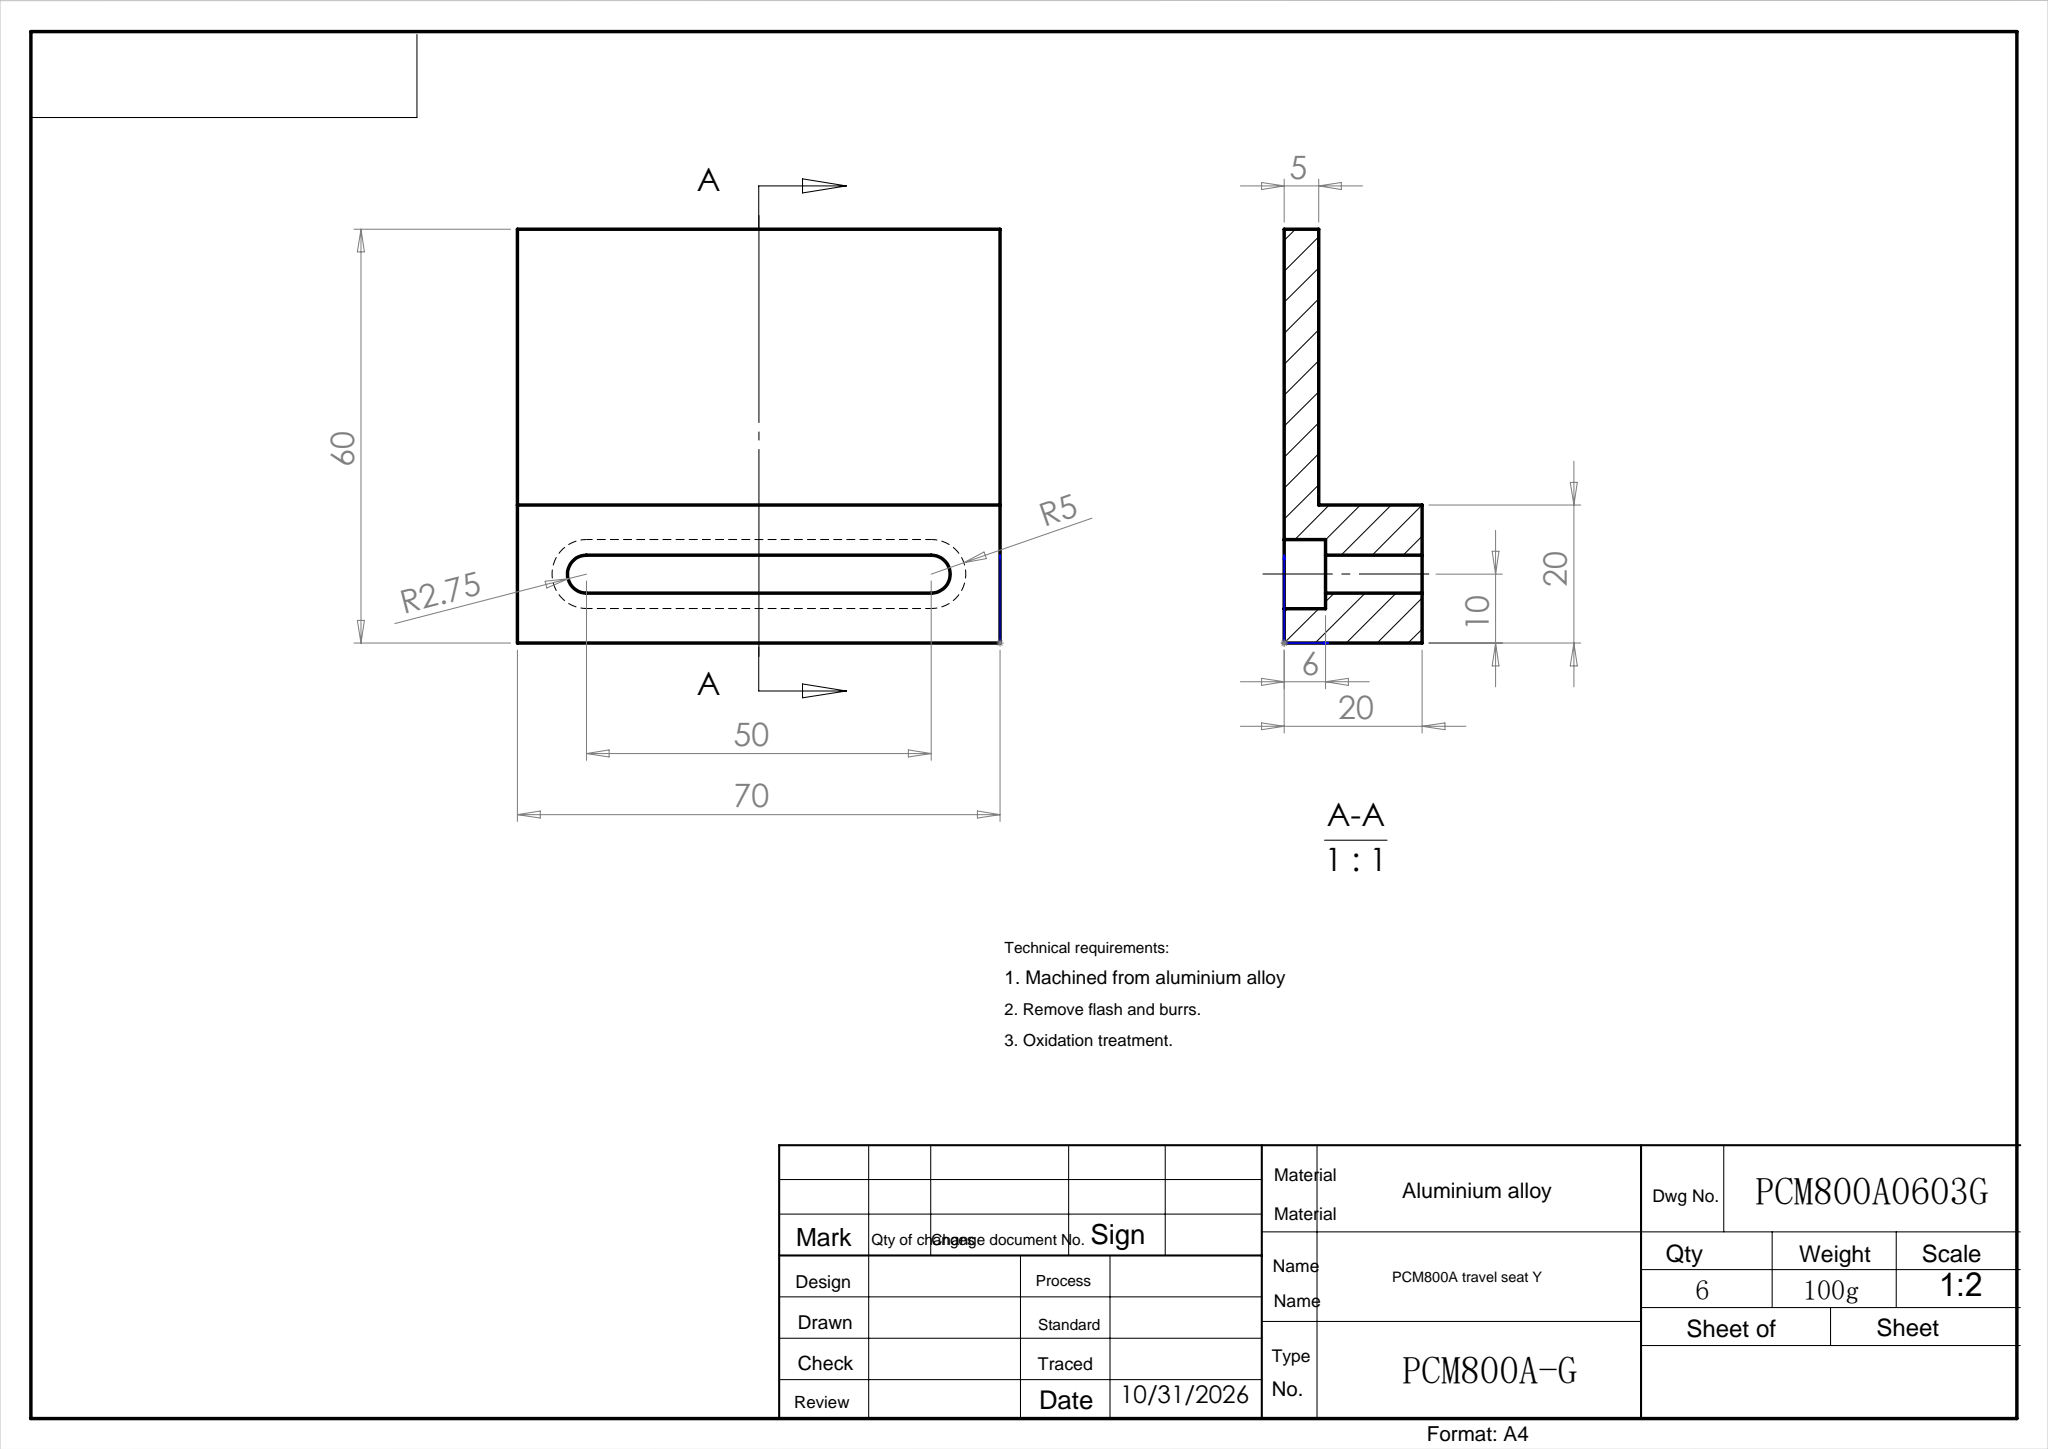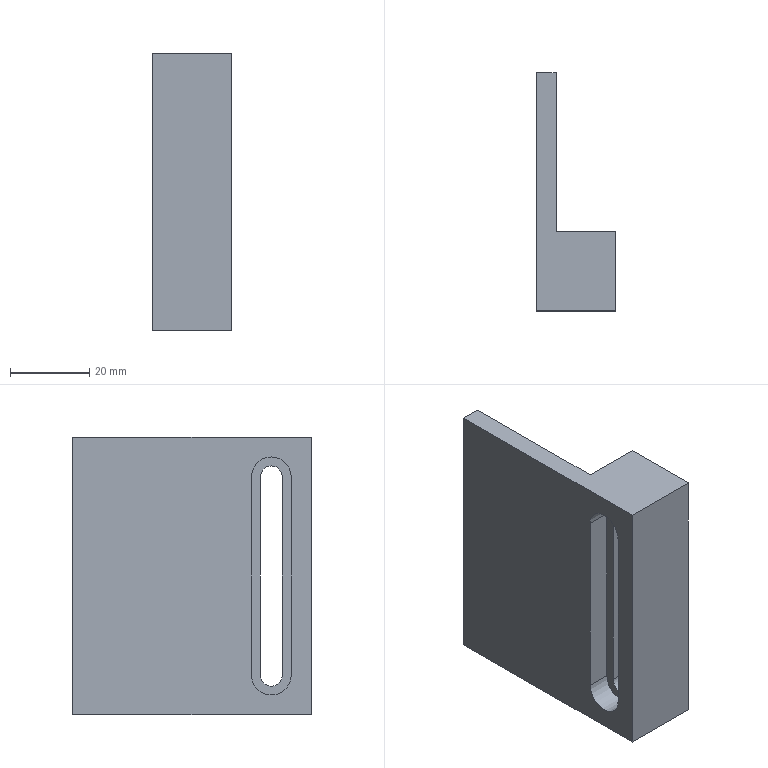Part | SolidWorks | features ICE 2, Extrusion 1 | 1 solid | 19 faces | box 20 x 60 x 70 mm | volume 34346 mm3 | plane 13 | cylinder 6 | commonest cylinder face diameters 5.5 x3 10 x3
STEP:
#1=CARTESIAN_POINT('',(6.,10.,65.));
#2=VERTEX_POINT('',#1);
#3=CARTESIAN_POINT('',(6.,15.,60.));
#4=VERTEX_POINT('',#3);
#5=CARTESIAN_POINT('',(6.,10.,60.));
#6=DIRECTION('',(-1.,0.,0.));
#7=DIRECTION('',(0.,0.,1.));
#8=AXIS2_PLACEMENT_3D('',#5,#6,#7);
#9=CIRCLE('',#8,5.);
#10=EDGE_CURVE('',#2,#4,#9,.T.);
#11=ORIENTED_EDGE('',*,*,#10,.F.);
#12=CARTESIAN_POINT('',(0.,10.,65.));
#13=VERTEX_POINT('',#12);
#14=CARTESIAN_POINT('',(6.,10.,65.));
#15=DIRECTION('',(-1.,0.,0.));
#16=VECTOR('',#15,1000.);
#17=LINE('',#14,#16);
#18=EDGE_CURVE('',#2,#13,#17,.T.);
#19=ORIENTED_EDGE('',*,*,#18,.T.);
#20=CARTESIAN_POINT('',(0.,15.,60.));
#21=VERTEX_POINT('',#20);
#22=CARTESIAN_POINT('',(0.,10.,60.));
#23=DIRECTION('',(-1.,0.,0.));
#24=DIRECTION('',(0.,0.,1.));
#25=AXIS2_PLACEMENT_3D('',#22,#23,#24);
#26=CIRCLE('',#25,5.);
#27=EDGE_CURVE('',#13,#21,#26,.T.);
#28=ORIENTED_EDGE('',*,*,#27,.T.);
#29=CARTESIAN_POINT('',(6.,15.,60.));
#30=DIRECTION('',(-1.,0.,0.));
#31=VECTOR('',#30,1000.);
#32=LINE('',#29,#31);
#33=EDGE_CURVE('',#4,#21,#32,.T.);
#34=ORIENTED_EDGE('',*,*,#33,.F.);
#35=EDGE_LOOP('',(#11,#19,#28,#34));
#36=FACE_OUTER_BOUND('',#35,.T.);
#37=CARTESIAN_POINT('',(6.,10.,60.));
#38=DIRECTION('',(-1.,0.,0.));
#39=DIRECTION('',(0.,0.,1.));
#40=AXIS2_PLACEMENT_3D('',#37,#38,#39);
#41=CYLINDRICAL_SURFACE('',#40,5.);
#42=ADVANCED_FACE('',(#36),#41,.F.);
#43=CARTESIAN_POINT('',(20.,10.,62.75));
#44=VERTEX_POINT('',#43);
#45=CARTESIAN_POINT('',(20.,12.75,60.));
#46=VERTEX_POINT('',#45);
#47=CARTESIAN_POINT('',(20.,10.,60.));
#48=DIRECTION('',(-1.,0.,0.));
#49=DIRECTION('',(0.,-1.,0.));
#50=AXIS2_PLACEMENT_3D('',#47,#48,#49);
#51=CIRCLE('',#50,2.75);
#52=EDGE_CURVE('',#44,#46,#51,.T.);
#53=ORIENTED_EDGE('',*,*,#52,.F.);
#54=CARTESIAN_POINT('',(6.,10.,62.75));
#55=VERTEX_POINT('',#54);
#56=CARTESIAN_POINT('',(1200.,10.,62.75));
#57=DIRECTION('',(-1.,0.,0.));
#58=VECTOR('',#57,1000.);
#59=LINE('',#56,#58);
#60=EDGE_CURVE('',#44,#55,#59,.T.);
#61=ORIENTED_EDGE('',*,*,#60,.T.);
#62=CARTESIAN_POINT('',(6.,12.75,60.));
#63=VERTEX_POINT('',#62);
#64=CARTESIAN_POINT('',(6.,10.,60.));
#65=DIRECTION('',(1.,0.,0.));
#66=DIRECTION('',(0.,0.,1.));
#67=AXIS2_PLACEMENT_3D('',#64,#65,#66);
#68=CIRCLE('',#67,2.75);
#69=EDGE_CURVE('',#63,#55,#68,.T.);
#70=ORIENTED_EDGE('',*,*,#69,.F.);
#71=CARTESIAN_POINT('',(1200.,12.75,60.));
#72=DIRECTION('',(-1.,0.,0.));
#73=VECTOR('',#72,1000.);
#74=LINE('',#71,#73);
#75=EDGE_CURVE('',#46,#63,#74,.T.);
#76=ORIENTED_EDGE('',*,*,#75,.F.);
#77=EDGE_LOOP('',(#53,#61,#70,#76));
#78=FACE_OUTER_BOUND('',#77,.T.);
#79=CARTESIAN_POINT('',(1200.,10.,60.));
#80=DIRECTION('',(-1.,0.,0.));
#81=DIRECTION('',(0.,0.,1.));
#82=AXIS2_PLACEMENT_3D('',#79,#80,#81);
#83=CYLINDRICAL_SURFACE('',#82,2.75);
#84=ADVANCED_FACE('',(#78),#83,.F.);
#85=CARTESIAN_POINT('',(6.,7.25,10.));
#86=VERTEX_POINT('',#85);
#87=CARTESIAN_POINT('',(6.,12.75,10.));
#88=VERTEX_POINT('',#87);
#89=CARTESIAN_POINT('',(6.,10.,10.));
#90=DIRECTION('',(1.,0.,0.));
#91=DIRECTION('',(0.,0.,1.));
#92=AXIS2_PLACEMENT_3D('',#89,#90,#91);
#93=CIRCLE('',#92,2.75);
#94=EDGE_CURVE('',#86,#88,#93,.T.);
#95=ORIENTED_EDGE('',*,*,#94,.F.);
#96=CARTESIAN_POINT('',(20.,7.25,10.));
#97=VERTEX_POINT('',#96);
#98=CARTESIAN_POINT('',(1200.,7.25,10.));
#99=DIRECTION('',(-1.,0.,0.));
#100=VECTOR('',#99,1000.);
#101=LINE('',#98,#100);
#102=EDGE_CURVE('',#97,#86,#101,.T.);
#103=ORIENTED_EDGE('',*,*,#102,.F.);
#104=CARTESIAN_POINT('',(20.,12.75,10.));
#105=VERTEX_POINT('',#104);
#106=CARTESIAN_POINT('',(20.,10.,10.));
#107=DIRECTION('',(-1.,0.,0.));
#108=DIRECTION('',(0.,-1.,0.));
#109=AXIS2_PLACEMENT_3D('',#106,#107,#108);
#110=CIRCLE('',#109,2.75);
#111=EDGE_CURVE('',#105,#97,#110,.T.);
#112=ORIENTED_EDGE('',*,*,#111,.F.);
#113=CARTESIAN_POINT('',(1200.,12.75,10.));
#114=DIRECTION('',(-1.,0.,0.));
#115=VECTOR('',#114,1000.);
#116=LINE('',#113,#115);
#117=EDGE_CURVE('',#105,#88,#116,.T.);
#118=ORIENTED_EDGE('',*,*,#117,.T.);
#119=EDGE_LOOP('',(#95,#103,#112,#118));
#120=FACE_OUTER_BOUND('',#119,.T.);
#121=CARTESIAN_POINT('',(1200.,10.,10.));
#122=DIRECTION('',(-1.,0.,0.));
#123=DIRECTION('',(0.,0.,1.));
#124=AXIS2_PLACEMENT_3D('',#121,#122,#123);
#125=CYLINDRICAL_SURFACE('',#124,2.75);
#126=ADVANCED_FACE('',(#120),#125,.F.);
#127=CARTESIAN_POINT('',(6.,12.75,10.));
#128=DIRECTION('',(0.,0.,1.));
#129=VECTOR('',#128,1000.);
#130=LINE('',#127,#129);
#131=EDGE_CURVE('',#88,#63,#130,.T.);
#132=ORIENTED_EDGE('',*,*,#131,.F.);
#133=ORIENTED_EDGE('',*,*,#117,.F.);
#134=CARTESIAN_POINT('',(20.,12.75,70.));
#135=DIRECTION('',(0.,0.,-1.));
#136=VECTOR('',#135,1000.);
#137=LINE('',#134,#136);
#138=EDGE_CURVE('',#46,#105,#137,.T.);
#139=ORIENTED_EDGE('',*,*,#138,.F.);
#140=ORIENTED_EDGE('',*,*,#75,.T.);
#141=EDGE_LOOP('',(#132,#133,#139,#140));
#142=FACE_OUTER_BOUND('',#141,.T.);
#143=CARTESIAN_POINT('',(1200.,12.75,10.));
#144=DIRECTION('',(0.,1.,0.));
#145=DIRECTION('',(0.,0.,1.));
#146=AXIS2_PLACEMENT_3D('',#143,#144,#145);
#147=PLANE('',#146);
#148=ADVANCED_FACE('',(#142),#147,.F.);
#149=ORIENTED_EDGE('',*,*,#60,.F.);
#150=CARTESIAN_POINT('',(20.,7.25,60.));
#151=VERTEX_POINT('',#150);
#152=CARTESIAN_POINT('',(20.,10.,60.));
#153=DIRECTION('',(-1.,0.,0.));
#154=DIRECTION('',(0.,-1.,0.));
#155=AXIS2_PLACEMENT_3D('',#152,#153,#154);
#156=CIRCLE('',#155,2.75);
#157=EDGE_CURVE('',#151,#44,#156,.T.);
#158=ORIENTED_EDGE('',*,*,#157,.F.);
#159=CARTESIAN_POINT('',(6.,7.25,60.));
#160=VERTEX_POINT('',#159);
#161=CARTESIAN_POINT('',(1200.,7.25,60.));
#162=DIRECTION('',(-1.,0.,0.));
#163=VECTOR('',#162,1000.);
#164=LINE('',#161,#163);
#165=EDGE_CURVE('',#151,#160,#164,.T.);
#166=ORIENTED_EDGE('',*,*,#165,.T.);
#167=CARTESIAN_POINT('',(6.,10.,60.));
#168=DIRECTION('',(1.,0.,0.));
#169=DIRECTION('',(0.,0.,1.));
#170=AXIS2_PLACEMENT_3D('',#167,#168,#169);
#171=CIRCLE('',#170,2.75);
#172=EDGE_CURVE('',#55,#160,#171,.T.);
#173=ORIENTED_EDGE('',*,*,#172,.F.);
#174=EDGE_LOOP('',(#149,#158,#166,#173));
#175=FACE_OUTER_BOUND('',#174,.T.);
#176=CARTESIAN_POINT('',(1200.,10.,60.));
#177=DIRECTION('',(-1.,0.,0.));
#178=DIRECTION('',(0.,0.,1.));
#179=AXIS2_PLACEMENT_3D('',#176,#177,#178);
#180=CYLINDRICAL_SURFACE('',#179,2.75);
#181=ADVANCED_FACE('',(#175),#180,.F.);
#182=CARTESIAN_POINT('',(6.,7.25,10.));
#183=DIRECTION('',(0.,0.,-1.));
#184=VECTOR('',#183,1000.);
#185=LINE('',#182,#184);
#186=EDGE_CURVE('',#160,#86,#185,.T.);
#187=ORIENTED_EDGE('',*,*,#186,.F.);
#188=ORIENTED_EDGE('',*,*,#165,.F.);
#189=CARTESIAN_POINT('',(20.,7.25,70.));
#190=DIRECTION('',(0.,0.,1.));
#191=VECTOR('',#190,1000.);
#192=LINE('',#189,#191);
#193=EDGE_CURVE('',#97,#151,#192,.T.);
#194=ORIENTED_EDGE('',*,*,#193,.F.);
#195=ORIENTED_EDGE('',*,*,#102,.T.);
#196=EDGE_LOOP('',(#187,#188,#194,#195));
#197=FACE_OUTER_BOUND('',#196,.T.);
#198=CARTESIAN_POINT('',(1200.,7.25,10.));
#199=DIRECTION('',(0.,-1.,0.));
#200=DIRECTION('',(0.,0.,-1.));
#201=AXIS2_PLACEMENT_3D('',#198,#199,#200);
#202=PLANE('',#201);
#203=ADVANCED_FACE('',(#197),#202,.F.);
#204=CARTESIAN_POINT('',(0.,0.,0.));
#205=VERTEX_POINT('',#204);
#206=CARTESIAN_POINT('',(20.,0.,0.));
#207=VERTEX_POINT('',#206);
#208=CARTESIAN_POINT('',(20.,0.,0.));
#209=DIRECTION('',(1.,0.,0.));
#210=VECTOR('',#209,1000.);
#211=LINE('',#208,#210);
#212=EDGE_CURVE('',#205,#207,#211,.T.);
#213=ORIENTED_EDGE('',*,*,#212,.T.);
#214=CARTESIAN_POINT('',(20.,0.,70.));
#215=VERTEX_POINT('',#214);
#216=CARTESIAN_POINT('',(20.,0.,70.));
#217=DIRECTION('',(0.,0.,-1.));
#218=VECTOR('',#217,1000.);
#219=LINE('',#216,#218);
#220=EDGE_CURVE('',#215,#207,#219,.T.);
#221=ORIENTED_EDGE('',*,*,#220,.F.);
#222=CARTESIAN_POINT('',(0.,0.,70.));
#223=VERTEX_POINT('',#222);
#224=CARTESIAN_POINT('',(20.,0.,70.));
#225=DIRECTION('',(1.,0.,0.));
#226=VECTOR('',#225,1000.);
#227=LINE('',#224,#226);
#228=EDGE_CURVE('',#223,#215,#227,.T.);
#229=ORIENTED_EDGE('',*,*,#228,.F.);
#230=CARTESIAN_POINT('',(0.,0.,70.));
#231=DIRECTION('',(0.,0.,-1.));
#232=VECTOR('',#231,1000.);
#233=LINE('',#230,#232);
#234=EDGE_CURVE('',#223,#205,#233,.T.);
#235=ORIENTED_EDGE('',*,*,#234,.T.);
#236=EDGE_LOOP('',(#213,#221,#229,#235));
#237=FACE_OUTER_BOUND('',#236,.T.);
#238=CARTESIAN_POINT('',(20.,0.,70.));
#239=DIRECTION('',(0.,1.,0.));
#240=DIRECTION('',(0.,0.,1.));
#241=AXIS2_PLACEMENT_3D('',#238,#239,#240);
#242=PLANE('',#241);
#243=ADVANCED_FACE('',(#237),#242,.F.);
#244=ORIENTED_EDGE('',*,*,#138,.T.);
#245=ORIENTED_EDGE('',*,*,#111,.T.);
#246=ORIENTED_EDGE('',*,*,#193,.T.);
#247=ORIENTED_EDGE('',*,*,#157,.T.);
#248=ORIENTED_EDGE('',*,*,#52,.T.);
#249=EDGE_LOOP('',(#244,#245,#246,#247,#248));
#250=FACE_BOUND('',#249,.T.);
#251=CARTESIAN_POINT('',(20.,20.,0.));
#252=VERTEX_POINT('',#251);
#253=CARTESIAN_POINT('',(20.,20.,0.));
#254=DIRECTION('',(0.,1.,0.));
#255=VECTOR('',#254,1000.);
#256=LINE('',#253,#255);
#257=EDGE_CURVE('',#207,#252,#256,.T.);
#258=ORIENTED_EDGE('',*,*,#257,.T.);
#259=CARTESIAN_POINT('',(20.,20.,70.));
#260=VERTEX_POINT('',#259);
#261=CARTESIAN_POINT('',(20.,20.,70.));
#262=DIRECTION('',(0.,0.,-1.));
#263=VECTOR('',#262,1000.);
#264=LINE('',#261,#263);
#265=EDGE_CURVE('',#260,#252,#264,.T.);
#266=ORIENTED_EDGE('',*,*,#265,.F.);
#267=CARTESIAN_POINT('',(20.,20.,70.));
#268=DIRECTION('',(0.,1.,0.));
#269=VECTOR('',#268,1000.);
#270=LINE('',#267,#269);
#271=EDGE_CURVE('',#215,#260,#270,.T.);
#272=ORIENTED_EDGE('',*,*,#271,.F.);
#273=ORIENTED_EDGE('',*,*,#220,.T.);
#274=EDGE_LOOP('',(#258,#266,#272,#273));
#275=FACE_OUTER_BOUND('',#274,.T.);
#276=CARTESIAN_POINT('',(20.,20.,70.));
#277=DIRECTION('',(-1.,0.,0.));
#278=DIRECTION('',(0.,-1.,0.));
#279=AXIS2_PLACEMENT_3D('',#276,#277,#278);
#280=PLANE('',#279);
#281=ADVANCED_FACE('',(#250,#275),#280,.F.);
#282=CARTESIAN_POINT('',(5.,20.,0.));
#283=VERTEX_POINT('',#282);
#284=CARTESIAN_POINT('',(5.,20.,0.));
#285=DIRECTION('',(-1.,0.,0.));
#286=VECTOR('',#285,1000.);
#287=LINE('',#284,#286);
#288=EDGE_CURVE('',#252,#283,#287,.T.);
#289=ORIENTED_EDGE('',*,*,#288,.T.);
#290=CARTESIAN_POINT('',(5.,20.,70.));
#291=VERTEX_POINT('',#290);
#292=CARTESIAN_POINT('',(5.,20.,70.));
#293=DIRECTION('',(0.,0.,-1.));
#294=VECTOR('',#293,1000.);
#295=LINE('',#292,#294);
#296=EDGE_CURVE('',#291,#283,#295,.T.);
#297=ORIENTED_EDGE('',*,*,#296,.F.);
#298=CARTESIAN_POINT('',(5.,20.,70.));
#299=DIRECTION('',(-1.,0.,0.));
#300=VECTOR('',#299,1000.);
#301=LINE('',#298,#300);
#302=EDGE_CURVE('',#260,#291,#301,.T.);
#303=ORIENTED_EDGE('',*,*,#302,.F.);
#304=ORIENTED_EDGE('',*,*,#265,.T.);
#305=EDGE_LOOP('',(#289,#297,#303,#304));
#306=FACE_OUTER_BOUND('',#305,.T.);
#307=CARTESIAN_POINT('',(5.,20.,70.));
#308=DIRECTION('',(0.,-1.,0.));
#309=DIRECTION('',(0.,0.,-1.));
#310=AXIS2_PLACEMENT_3D('',#307,#308,#309);
#311=PLANE('',#310);
#312=ADVANCED_FACE('',(#306),#311,.F.);
#313=CARTESIAN_POINT('',(5.,60.,0.));
#314=VERTEX_POINT('',#313);
#315=CARTESIAN_POINT('',(5.,60.,0.));
#316=DIRECTION('',(0.,1.,0.));
#317=VECTOR('',#316,1000.);
#318=LINE('',#315,#317);
#319=EDGE_CURVE('',#283,#314,#318,.T.);
#320=ORIENTED_EDGE('',*,*,#319,.T.);
#321=CARTESIAN_POINT('',(5.,60.,70.));
#322=VERTEX_POINT('',#321);
#323=CARTESIAN_POINT('',(5.,60.,70.));
#324=DIRECTION('',(0.,0.,-1.));
#325=VECTOR('',#324,1000.);
#326=LINE('',#323,#325);
#327=EDGE_CURVE('',#322,#314,#326,.T.);
#328=ORIENTED_EDGE('',*,*,#327,.F.);
#329=CARTESIAN_POINT('',(5.,60.,70.));
#330=DIRECTION('',(0.,1.,0.));
#331=VECTOR('',#330,1000.);
#332=LINE('',#329,#331);
#333=EDGE_CURVE('',#291,#322,#332,.T.);
#334=ORIENTED_EDGE('',*,*,#333,.F.);
#335=ORIENTED_EDGE('',*,*,#296,.T.);
#336=EDGE_LOOP('',(#320,#328,#334,#335));
#337=FACE_OUTER_BOUND('',#336,.T.);
#338=CARTESIAN_POINT('',(5.,60.,70.));
#339=DIRECTION('',(-1.,0.,0.));
#340=DIRECTION('',(0.,-1.,0.));
#341=AXIS2_PLACEMENT_3D('',#338,#339,#340);
#342=PLANE('',#341);
#343=ADVANCED_FACE('',(#337),#342,.F.);
#344=CARTESIAN_POINT('',(0.,60.,0.));
#345=VERTEX_POINT('',#344);
#346=CARTESIAN_POINT('',(0.,60.,0.));
#347=DIRECTION('',(-1.,0.,0.));
#348=VECTOR('',#347,1000.);
#349=LINE('',#346,#348);
#350=EDGE_CURVE('',#314,#345,#349,.T.);
#351=ORIENTED_EDGE('',*,*,#350,.T.);
#352=CARTESIAN_POINT('',(0.,60.,70.));
#353=VERTEX_POINT('',#352);
#354=CARTESIAN_POINT('',(0.,60.,70.));
#355=DIRECTION('',(0.,0.,-1.));
#356=VECTOR('',#355,1000.);
#357=LINE('',#354,#356);
#358=EDGE_CURVE('',#353,#345,#357,.T.);
#359=ORIENTED_EDGE('',*,*,#358,.F.);
#360=CARTESIAN_POINT('',(0.,60.,70.));
#361=DIRECTION('',(-1.,0.,0.));
#362=VECTOR('',#361,1000.);
#363=LINE('',#360,#362);
#364=EDGE_CURVE('',#322,#353,#363,.T.);
#365=ORIENTED_EDGE('',*,*,#364,.F.);
#366=ORIENTED_EDGE('',*,*,#327,.T.);
#367=EDGE_LOOP('',(#351,#359,#365,#366));
#368=FACE_OUTER_BOUND('',#367,.T.);
#369=CARTESIAN_POINT('',(0.,60.,70.));
#370=DIRECTION('',(0.,-1.,0.));
#371=DIRECTION('',(0.,0.,-1.));
#372=AXIS2_PLACEMENT_3D('',#369,#370,#371);
#373=PLANE('',#372);
#374=ADVANCED_FACE('',(#368),#373,.F.);
#375=CARTESIAN_POINT('',(0.,5.,10.));
#376=VERTEX_POINT('',#375);
#377=CARTESIAN_POINT('',(0.,5.,60.));
#378=VERTEX_POINT('',#377);
#379=CARTESIAN_POINT('',(0.,5.,10.));
#380=DIRECTION('',(0.,0.,1.));
#381=VECTOR('',#380,1000.);
#382=LINE('',#379,#381);
#383=EDGE_CURVE('',#376,#378,#382,.T.);
#384=ORIENTED_EDGE('',*,*,#383,.F.);
#385=CARTESIAN_POINT('',(0.,15.,10.));
#386=VERTEX_POINT('',#385);
#387=CARTESIAN_POINT('',(0.,10.,10.));
#388=DIRECTION('',(-1.,0.,0.));
#389=DIRECTION('',(0.,0.,1.));
#390=AXIS2_PLACEMENT_3D('',#387,#388,#389);
#391=CIRCLE('',#390,5.);
#392=EDGE_CURVE('',#386,#376,#391,.T.);
#393=ORIENTED_EDGE('',*,*,#392,.F.);
#394=CARTESIAN_POINT('',(0.,15.,60.));
#395=DIRECTION('',(0.,0.,-1.));
#396=VECTOR('',#395,1000.);
#397=LINE('',#394,#396);
#398=EDGE_CURVE('',#21,#386,#397,.T.);
#399=ORIENTED_EDGE('',*,*,#398,.F.);
#400=ORIENTED_EDGE('',*,*,#27,.F.);
#401=CARTESIAN_POINT('',(0.,10.,60.));
#402=DIRECTION('',(-1.,0.,0.));
#403=DIRECTION('',(0.,0.,1.));
#404=AXIS2_PLACEMENT_3D('',#401,#402,#403);
#405=CIRCLE('',#404,5.);
#406=EDGE_CURVE('',#378,#13,#405,.T.);
#407=ORIENTED_EDGE('',*,*,#406,.F.);
#408=EDGE_LOOP('',(#384,#393,#399,#400,#407));
#409=FACE_BOUND('',#408,.T.);
#410=CARTESIAN_POINT('',(0.,0.,0.));
#411=DIRECTION('',(0.,-1.,0.));
#412=VECTOR('',#411,1000.);
#413=LINE('',#410,#412);
#414=EDGE_CURVE('',#345,#205,#413,.T.);
#415=ORIENTED_EDGE('',*,*,#414,.T.);
#416=ORIENTED_EDGE('',*,*,#234,.F.);
#417=CARTESIAN_POINT('',(0.,0.,70.));
#418=DIRECTION('',(0.,-1.,0.));
#419=VECTOR('',#418,1000.);
#420=LINE('',#417,#419);
#421=EDGE_CURVE('',#353,#223,#420,.T.);
#422=ORIENTED_EDGE('',*,*,#421,.F.);
#423=ORIENTED_EDGE('',*,*,#358,.T.);
#424=EDGE_LOOP('',(#415,#416,#422,#423));
#425=FACE_OUTER_BOUND('',#424,.T.);
#426=CARTESIAN_POINT('',(0.,0.,70.));
#427=DIRECTION('',(1.,0.,0.));
#428=DIRECTION('',(0.,0.,-1.));
#429=AXIS2_PLACEMENT_3D('',#426,#427,#428);
#430=PLANE('',#429);
#431=ADVANCED_FACE('',(#409,#425),#430,.F.);
#432=ORIENTED_EDGE('',*,*,#228,.T.);
#433=ORIENTED_EDGE('',*,*,#271,.T.);
#434=ORIENTED_EDGE('',*,*,#302,.T.);
#435=ORIENTED_EDGE('',*,*,#333,.T.);
#436=ORIENTED_EDGE('',*,*,#364,.T.);
#437=ORIENTED_EDGE('',*,*,#421,.T.);
#438=EDGE_LOOP('',(#432,#433,#434,#435,#436,#437));
#439=FACE_OUTER_BOUND('',#438,.T.);
#440=CARTESIAN_POINT('',(0.,0.,70.));
#441=DIRECTION('',(0.,0.,-1.));
#442=DIRECTION('',(-1.,0.,0.));
#443=AXIS2_PLACEMENT_3D('',#440,#441,#442);
#444=PLANE('',#443);
#445=ADVANCED_FACE('',(#439),#444,.F.);
#446=ORIENTED_EDGE('',*,*,#212,.F.);
#447=ORIENTED_EDGE('',*,*,#414,.F.);
#448=ORIENTED_EDGE('',*,*,#350,.F.);
#449=ORIENTED_EDGE('',*,*,#319,.F.);
#450=ORIENTED_EDGE('',*,*,#288,.F.);
#451=ORIENTED_EDGE('',*,*,#257,.F.);
#452=EDGE_LOOP('',(#446,#447,#448,#449,#450,#451));
#453=FACE_OUTER_BOUND('',#452,.T.);
#454=CARTESIAN_POINT('',(0.,0.,0.));
#455=DIRECTION('',(0.,0.,-1.));
#456=DIRECTION('',(-1.,0.,0.));
#457=AXIS2_PLACEMENT_3D('',#454,#455,#456);
#458=PLANE('',#457);
#459=ADVANCED_FACE('',(#453),#458,.T.);
#460=CARTESIAN_POINT('',(6.,15.,10.));
#461=VERTEX_POINT('',#460);
#462=CARTESIAN_POINT('',(6.,5.,10.));
#463=VERTEX_POINT('',#462);
#464=CARTESIAN_POINT('',(6.,10.,10.));
#465=DIRECTION('',(-1.,0.,0.));
#466=DIRECTION('',(0.,0.,1.));
#467=AXIS2_PLACEMENT_3D('',#464,#465,#466);
#468=CIRCLE('',#467,5.);
#469=EDGE_CURVE('',#461,#463,#468,.T.);
#470=ORIENTED_EDGE('',*,*,#469,.T.);
#471=CARTESIAN_POINT('',(6.,5.,60.));
#472=VERTEX_POINT('',#471);
#473=CARTESIAN_POINT('',(6.,5.,10.));
#474=DIRECTION('',(0.,0.,1.));
#475=VECTOR('',#474,1000.);
#476=LINE('',#473,#475);
#477=EDGE_CURVE('',#463,#472,#476,.T.);
#478=ORIENTED_EDGE('',*,*,#477,.T.);
#479=CARTESIAN_POINT('',(6.,10.,60.));
#480=DIRECTION('',(-1.,0.,0.));
#481=DIRECTION('',(0.,0.,1.));
#482=AXIS2_PLACEMENT_3D('',#479,#480,#481);
#483=CIRCLE('',#482,5.);
#484=EDGE_CURVE('',#472,#2,#483,.T.);
#485=ORIENTED_EDGE('',*,*,#484,.T.);
#486=ORIENTED_EDGE('',*,*,#10,.T.);
#487=CARTESIAN_POINT('',(6.,15.,60.));
#488=DIRECTION('',(0.,0.,-1.));
#489=VECTOR('',#488,1000.);
#490=LINE('',#487,#489);
#491=EDGE_CURVE('',#4,#461,#490,.T.);
#492=ORIENTED_EDGE('',*,*,#491,.T.);
#493=EDGE_LOOP('',(#470,#478,#485,#486,#492));
#494=FACE_OUTER_BOUND('',#493,.T.);
#495=ORIENTED_EDGE('',*,*,#94,.T.);
#496=ORIENTED_EDGE('',*,*,#131,.T.);
#497=ORIENTED_EDGE('',*,*,#69,.T.);
#498=ORIENTED_EDGE('',*,*,#172,.T.);
#499=ORIENTED_EDGE('',*,*,#186,.T.);
#500=EDGE_LOOP('',(#495,#496,#497,#498,#499));
#501=FACE_BOUND('',#500,.T.);
#502=CARTESIAN_POINT('',(6.,10.,10.));
#503=DIRECTION('',(-1.,0.,0.));
#504=DIRECTION('',(0.,0.,1.));
#505=AXIS2_PLACEMENT_3D('',#502,#503,#504);
#506=PLANE('',#505);
#507=ADVANCED_FACE('',(#494,#501),#506,.T.);
#508=ORIENTED_EDGE('',*,*,#392,.T.);
#509=CARTESIAN_POINT('',(6.,5.,10.));
#510=DIRECTION('',(-1.,0.,0.));
#511=VECTOR('',#510,1000.);
#512=LINE('',#509,#511);
#513=EDGE_CURVE('',#463,#376,#512,.T.);
#514=ORIENTED_EDGE('',*,*,#513,.F.);
#515=ORIENTED_EDGE('',*,*,#469,.F.);
#516=CARTESIAN_POINT('',(6.,15.,10.));
#517=DIRECTION('',(-1.,0.,0.));
#518=VECTOR('',#517,1000.);
#519=LINE('',#516,#518);
#520=EDGE_CURVE('',#461,#386,#519,.T.);
#521=ORIENTED_EDGE('',*,*,#520,.T.);
#522=EDGE_LOOP('',(#508,#514,#515,#521));
#523=FACE_OUTER_BOUND('',#522,.T.);
#524=CARTESIAN_POINT('',(6.,10.,10.));
#525=DIRECTION('',(-1.,0.,0.));
#526=DIRECTION('',(0.,0.,1.));
#527=AXIS2_PLACEMENT_3D('',#524,#525,#526);
#528=CYLINDRICAL_SURFACE('',#527,5.);
#529=ADVANCED_FACE('',(#523),#528,.F.);
#530=ORIENTED_EDGE('',*,*,#398,.T.);
#531=ORIENTED_EDGE('',*,*,#520,.F.);
#532=ORIENTED_EDGE('',*,*,#491,.F.);
#533=ORIENTED_EDGE('',*,*,#33,.T.);
#534=EDGE_LOOP('',(#530,#531,#532,#533));
#535=FACE_OUTER_BOUND('',#534,.T.);
#536=CARTESIAN_POINT('',(6.,15.,60.));
#537=DIRECTION('',(0.,1.,0.));
#538=DIRECTION('',(0.,0.,1.));
#539=AXIS2_PLACEMENT_3D('',#536,#537,#538);
#540=PLANE('',#539);
#541=ADVANCED_FACE('',(#535),#540,.F.);
#542=ORIENTED_EDGE('',*,*,#18,.F.);
#543=ORIENTED_EDGE('',*,*,#484,.F.);
#544=CARTESIAN_POINT('',(6.,5.,60.));
#545=DIRECTION('',(-1.,0.,0.));
#546=VECTOR('',#545,1000.);
#547=LINE('',#544,#546);
#548=EDGE_CURVE('',#472,#378,#547,.T.);
#549=ORIENTED_EDGE('',*,*,#548,.T.);
#550=ORIENTED_EDGE('',*,*,#406,.T.);
#551=EDGE_LOOP('',(#542,#543,#549,#550));
#552=FACE_OUTER_BOUND('',#551,.T.);
#553=CARTESIAN_POINT('',(6.,10.,60.));
#554=DIRECTION('',(-1.,0.,0.));
#555=DIRECTION('',(0.,0.,1.));
#556=AXIS2_PLACEMENT_3D('',#553,#554,#555);
#557=CYLINDRICAL_SURFACE('',#556,5.);
#558=ADVANCED_FACE('',(#552),#557,.F.);
#559=ORIENTED_EDGE('',*,*,#383,.T.);
#560=ORIENTED_EDGE('',*,*,#548,.F.);
#561=ORIENTED_EDGE('',*,*,#477,.F.);
#562=ORIENTED_EDGE('',*,*,#513,.T.);
#563=EDGE_LOOP('',(#559,#560,#561,#562));
#564=FACE_OUTER_BOUND('',#563,.T.);
#565=CARTESIAN_POINT('',(6.,5.,10.));
#566=DIRECTION('',(0.,-1.,0.));
#567=DIRECTION('',(0.,0.,-1.));
#568=AXIS2_PLACEMENT_3D('',#565,#566,#567);
#569=PLANE('',#568);
#570=ADVANCED_FACE('',(#564),#569,.F.);
#571=CLOSED_SHELL('',(#42,#84,#126,#148,#181,#203,#243,#281,#312,#343,#374,#431,#445,#459,#507,#529,#541,#558,#570));
#572=MANIFOLD_SOLID_BREP('',#571);
#573=CARTESIAN_POINT('',(0.,0.,0.));
#574=DIRECTION('',(0.,0.,1.));
#575=DIRECTION('',(1.,0.,0.));
#576=AXIS2_PLACEMENT_3D('',#573,#574,#575);
#577=(LENGTH_UNIT()NAMED_UNIT(*)SI_UNIT(.MILLI.,.METRE.));
#578=UNCERTAINTY_MEASURE_WITH_UNIT(LENGTH_MEASURE(0.00001),#577,'','');
#579=(NAMED_UNIT(*)PLANE_ANGLE_UNIT()SI_UNIT($,.RADIAN.));
#580=(NAMED_UNIT(*)SI_UNIT($,.STERADIAN.)SOLID_ANGLE_UNIT());
#581=(GEOMETRIC_REPRESENTATION_CONTEXT(3)GLOBAL_UNCERTAINTY_ASSIGNED_CONTEXT((#578))GLOBAL_UNIT_ASSIGNED_CONTEXT((#577,#579,#580))REPRESENTATION_CONTEXT('',''));
#582=ADVANCED_BREP_SHAPE_REPRESENTATION('',(#572,#576),#581);